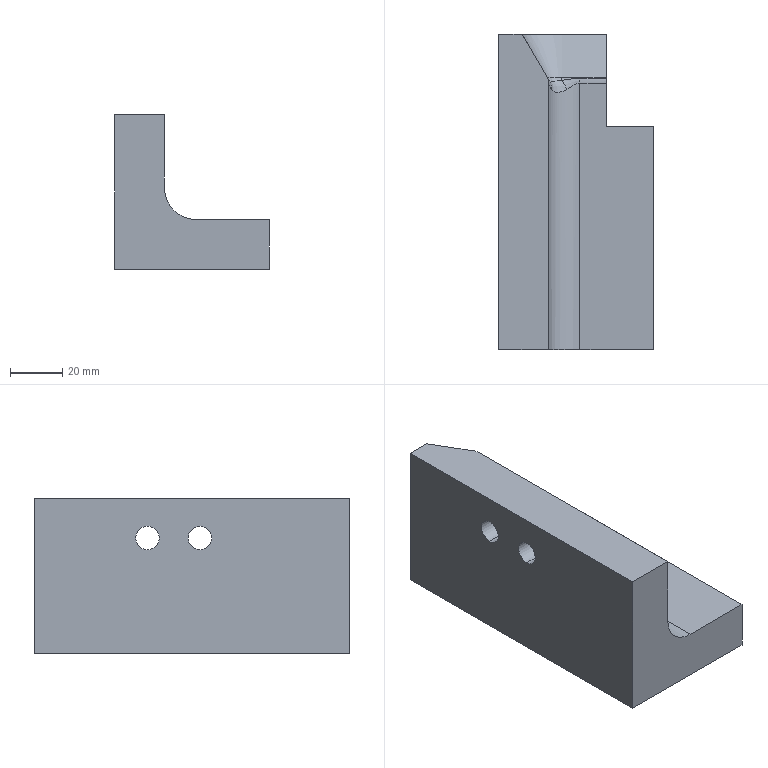Part | 1 solid | 30 faces | box 59 x 120 x 59.001 mm | volume 206950 mm3 | cylinder 13 | plane 12 | spline 5 | commonest cylinder face diameters 9 x4 15 x4 4 x2 10 x2 24 x1
STEP:
#1=CARTESIAN_POINT('',(-19.,-25.,120.5));
#2=VERTEX_POINT('',#1);
#3=CARTESIAN_POINT('',(-19.,-25.,105.5));
#4=VERTEX_POINT('',#3);
#5=CARTESIAN_POINT('',(-19.,-25.,113.));
#6=DIRECTION('',(-1.,0.,0.));
#7=DIRECTION('',(0.,0.,1.));
#8=AXIS2_PLACEMENT_3D('',#5,#6,#7);
#9=CIRCLE('',#8,7.5);
#10=EDGE_CURVE('',#2,#4,#9,.T.);
#11=ORIENTED_EDGE('',*,*,#10,.T.);
#12=CARTESIAN_POINT('',(-10.,-25.,105.5));
#13=VERTEX_POINT('',#12);
#14=CARTESIAN_POINT('',(-10.,-25.,105.5));
#15=DIRECTION('',(1.,0.,0.));
#16=VECTOR('',#15,1000.);
#17=LINE('',#14,#16);
#18=EDGE_CURVE('',#4,#13,#17,.T.);
#19=ORIENTED_EDGE('',*,*,#18,.T.);
#20=CARTESIAN_POINT('',(-10.,-25.,120.5));
#21=VERTEX_POINT('',#20);
#22=CARTESIAN_POINT('',(-10.,-25.,113.));
#23=DIRECTION('',(-1.,0.,0.));
#24=DIRECTION('',(0.,0.,1.));
#25=AXIS2_PLACEMENT_3D('',#22,#23,#24);
#26=CIRCLE('',#25,7.5);
#27=EDGE_CURVE('',#21,#13,#26,.T.);
#28=ORIENTED_EDGE('',*,*,#27,.F.);
#29=CARTESIAN_POINT('',(-10.,-25.,120.5));
#30=DIRECTION('',(1.,0.,0.));
#31=VECTOR('',#30,1000.);
#32=LINE('',#29,#31);
#33=EDGE_CURVE('',#2,#21,#32,.T.);
#34=ORIENTED_EDGE('',*,*,#33,.F.);
#35=EDGE_LOOP('',(#11,#19,#28,#34));
#36=FACE_OUTER_BOUND('',#35,.T.);
#37=CARTESIAN_POINT('',(-10.,-25.,113.));
#38=DIRECTION('',(1.,0.,0.));
#39=DIRECTION('',(0.,0.,1.));
#40=AXIS2_PLACEMENT_3D('',#37,#38,#39);
#41=CYLINDRICAL_SURFACE('',#40,7.5);
#42=ADVANCED_FACE('',(#36),#41,.F.);
#43=CARTESIAN_POINT('',(-19.,-45.,120.5));
#44=VERTEX_POINT('',#43);
#45=CARTESIAN_POINT('',(-19.,-45.,105.5));
#46=VERTEX_POINT('',#45);
#47=CARTESIAN_POINT('',(-19.,-45.,113.));
#48=DIRECTION('',(-1.,0.,0.));
#49=DIRECTION('',(0.,0.,1.));
#50=AXIS2_PLACEMENT_3D('',#47,#48,#49);
#51=CIRCLE('',#50,7.5);
#52=EDGE_CURVE('',#44,#46,#51,.T.);
#53=ORIENTED_EDGE('',*,*,#52,.T.);
#54=CARTESIAN_POINT('',(-10.,-45.,105.5));
#55=VERTEX_POINT('',#54);
#56=CARTESIAN_POINT('',(-10.,-45.,105.5));
#57=DIRECTION('',(1.,0.,0.));
#58=VECTOR('',#57,1000.);
#59=LINE('',#56,#58);
#60=EDGE_CURVE('',#46,#55,#59,.T.);
#61=ORIENTED_EDGE('',*,*,#60,.T.);
#62=CARTESIAN_POINT('',(-10.,-45.,120.5));
#63=VERTEX_POINT('',#62);
#64=CARTESIAN_POINT('',(-10.,-45.,113.));
#65=DIRECTION('',(-1.,0.,0.));
#66=DIRECTION('',(0.,0.,1.));
#67=AXIS2_PLACEMENT_3D('',#64,#65,#66);
#68=CIRCLE('',#67,7.5);
#69=EDGE_CURVE('',#63,#55,#68,.T.);
#70=ORIENTED_EDGE('',*,*,#69,.F.);
#71=CARTESIAN_POINT('',(-10.,-45.,120.5));
#72=DIRECTION('',(1.,0.,0.));
#73=VECTOR('',#72,1000.);
#74=LINE('',#71,#73);
#75=EDGE_CURVE('',#44,#63,#74,.T.);
#76=ORIENTED_EDGE('',*,*,#75,.F.);
#77=EDGE_LOOP('',(#53,#61,#70,#76));
#78=FACE_OUTER_BOUND('',#77,.T.);
#79=CARTESIAN_POINT('',(-10.,-45.,113.));
#80=DIRECTION('',(1.,0.,0.));
#81=DIRECTION('',(0.,0.,1.));
#82=AXIS2_PLACEMENT_3D('',#79,#80,#81);
#83=CYLINDRICAL_SURFACE('',#82,7.5);
#84=ADVANCED_FACE('',(#78),#83,.F.);
#85=CARTESIAN_POINT('',(-29.,-25.,117.5));
#86=VERTEX_POINT('',#85);
#87=CARTESIAN_POINT('',(-29.,-25.,108.5));
#88=VERTEX_POINT('',#87);
#89=CARTESIAN_POINT('',(-29.,-25.,113.));
#90=DIRECTION('',(-1.,0.,0.));
#91=DIRECTION('',(0.,0.,-1.));
#92=AXIS2_PLACEMENT_3D('',#89,#90,#91);
#93=CIRCLE('',#92,4.5);
#94=EDGE_CURVE('',#86,#88,#93,.T.);
#95=ORIENTED_EDGE('',*,*,#94,.T.);
#96=CARTESIAN_POINT('',(-19.,-25.,108.5));
#97=VERTEX_POINT('',#96);
#98=CARTESIAN_POINT('',(-10.,-25.,108.5));
#99=DIRECTION('',(1.,0.,0.));
#100=VECTOR('',#99,1000.);
#101=LINE('',#98,#100);
#102=EDGE_CURVE('',#88,#97,#101,.T.);
#103=ORIENTED_EDGE('',*,*,#102,.T.);
#104=CARTESIAN_POINT('',(-19.,-25.,117.5));
#105=VERTEX_POINT('',#104);
#106=CARTESIAN_POINT('',(-19.,-25.,113.));
#107=DIRECTION('',(-1.,0.,0.));
#108=DIRECTION('',(0.,0.,1.));
#109=AXIS2_PLACEMENT_3D('',#106,#107,#108);
#110=CIRCLE('',#109,4.5);
#111=EDGE_CURVE('',#105,#97,#110,.T.);
#112=ORIENTED_EDGE('',*,*,#111,.F.);
#113=CARTESIAN_POINT('',(-10.,-25.,117.5));
#114=DIRECTION('',(1.,0.,0.));
#115=VECTOR('',#114,1000.);
#116=LINE('',#113,#115);
#117=EDGE_CURVE('',#86,#105,#116,.T.);
#118=ORIENTED_EDGE('',*,*,#117,.F.);
#119=EDGE_LOOP('',(#95,#103,#112,#118));
#120=FACE_OUTER_BOUND('',#119,.T.);
#121=CARTESIAN_POINT('',(-10.,-25.,113.));
#122=DIRECTION('',(1.,0.,0.));
#123=DIRECTION('',(0.,0.,1.));
#124=AXIS2_PLACEMENT_3D('',#121,#122,#123);
#125=CYLINDRICAL_SURFACE('',#124,4.5);
#126=ADVANCED_FACE('',(#120),#125,.F.);
#127=CARTESIAN_POINT('',(-29.,-45.,117.5));
#128=VERTEX_POINT('',#127);
#129=CARTESIAN_POINT('',(-29.,-45.,108.5));
#130=VERTEX_POINT('',#129);
#131=CARTESIAN_POINT('',(-29.,-45.,113.));
#132=DIRECTION('',(-1.,0.,0.));
#133=DIRECTION('',(0.,0.,-1.));
#134=AXIS2_PLACEMENT_3D('',#131,#132,#133);
#135=CIRCLE('',#134,4.5);
#136=EDGE_CURVE('',#128,#130,#135,.T.);
#137=ORIENTED_EDGE('',*,*,#136,.T.);
#138=CARTESIAN_POINT('',(-19.,-45.,108.5));
#139=VERTEX_POINT('',#138);
#140=CARTESIAN_POINT('',(-10.,-45.,108.5));
#141=DIRECTION('',(1.,0.,0.));
#142=VECTOR('',#141,1000.);
#143=LINE('',#140,#142);
#144=EDGE_CURVE('',#130,#139,#143,.T.);
#145=ORIENTED_EDGE('',*,*,#144,.T.);
#146=CARTESIAN_POINT('',(-19.,-45.,117.5));
#147=VERTEX_POINT('',#146);
#148=CARTESIAN_POINT('',(-19.,-45.,113.));
#149=DIRECTION('',(-1.,0.,0.));
#150=DIRECTION('',(0.,0.,1.));
#151=AXIS2_PLACEMENT_3D('',#148,#149,#150);
#152=CIRCLE('',#151,4.5);
#153=EDGE_CURVE('',#147,#139,#152,.T.);
#154=ORIENTED_EDGE('',*,*,#153,.F.);
#155=CARTESIAN_POINT('',(-10.,-45.,117.5));
#156=DIRECTION('',(1.,0.,0.));
#157=VECTOR('',#156,1000.);
#158=LINE('',#155,#157);
#159=EDGE_CURVE('',#128,#147,#158,.T.);
#160=ORIENTED_EDGE('',*,*,#159,.F.);
#161=EDGE_LOOP('',(#137,#145,#154,#160));
#162=FACE_OUTER_BOUND('',#161,.T.);
#163=CARTESIAN_POINT('',(-10.,-45.,113.));
#164=DIRECTION('',(1.,0.,0.));
#165=DIRECTION('',(0.,0.,1.));
#166=AXIS2_PLACEMENT_3D('',#163,#164,#165);
#167=CYLINDRICAL_SURFACE('',#166,4.5);
#168=ADVANCED_FACE('',(#162),#167,.F.);
#169=CARTESIAN_POINT('',(-29.,-102.,69.));
#170=VERTEX_POINT('',#169);
#171=CARTESIAN_POINT('',(30.,-102.,69.));
#172=VERTEX_POINT('',#171);
#173=CARTESIAN_POINT('',(-30.,-102.,69.));
#174=DIRECTION('',(1.,0.,0.));
#175=VECTOR('',#174,1000.);
#176=LINE('',#173,#175);
#177=EDGE_CURVE('',#170,#172,#176,.T.);
#178=ORIENTED_EDGE('',*,*,#177,.T.);
#179=CARTESIAN_POINT('',(30.,-102.,88.));
#180=VERTEX_POINT('',#179);
#181=CARTESIAN_POINT('',(30.,-102.,88.));
#182=DIRECTION('',(0.,0.,-1.));
#183=VECTOR('',#182,1000.);
#184=LINE('',#181,#183);
#185=EDGE_CURVE('',#180,#172,#184,.T.);
#186=ORIENTED_EDGE('',*,*,#185,.F.);
#187=CARTESIAN_POINT('',(2.,-102.,88.));
#188=VERTEX_POINT('',#187);
#189=CARTESIAN_POINT('',(2.,-102.,88.));
#190=DIRECTION('',(1.,0.,0.));
#191=VECTOR('',#190,1000.);
#192=LINE('',#189,#191);
#193=EDGE_CURVE('',#188,#180,#192,.T.);
#194=ORIENTED_EDGE('',*,*,#193,.F.);
#195=CARTESIAN_POINT('',(-10.,-102.,100.));
#196=VERTEX_POINT('',#195);
#197=CARTESIAN_POINT('',(2.,-102.,100.));
#198=DIRECTION('',(0.,-1.,0.));
#199=DIRECTION('',(0.,0.,1.));
#200=AXIS2_PLACEMENT_3D('',#197,#198,#199);
#201=CIRCLE('',#200,12.);
#202=EDGE_CURVE('',#196,#188,#201,.T.);
#203=ORIENTED_EDGE('',*,*,#202,.F.);
#204=CARTESIAN_POINT('',(-10.,-102.,128.));
#205=VERTEX_POINT('',#204);
#206=CARTESIAN_POINT('',(-10.,-102.,128.));
#207=DIRECTION('',(0.,0.,-1.));
#208=VECTOR('',#207,1000.);
#209=LINE('',#206,#208);
#210=EDGE_CURVE('',#205,#196,#209,.T.);
#211=ORIENTED_EDGE('',*,*,#210,.F.);
#212=CARTESIAN_POINT('',(-29.,-102.,128.));
#213=VERTEX_POINT('',#212);
#214=CARTESIAN_POINT('',(-30.,-102.,128.));
#215=DIRECTION('',(1.,0.,0.));
#216=VECTOR('',#215,1000.);
#217=LINE('',#214,#216);
#218=EDGE_CURVE('',#213,#205,#217,.T.);
#219=ORIENTED_EDGE('',*,*,#218,.F.);
#220=CARTESIAN_POINT('',(-29.,-102.,128.));
#221=DIRECTION('',(0.,0.,-1.));
#222=VECTOR('',#221,1000.);
#223=LINE('',#220,#222);
#224=EDGE_CURVE('',#213,#170,#223,.T.);
#225=ORIENTED_EDGE('',*,*,#224,.T.);
#226=EDGE_LOOP('',(#178,#186,#194,#203,#211,#219,#225));
#227=FACE_OUTER_BOUND('',#226,.T.);
#228=CARTESIAN_POINT('',(2.,-102.,100.));
#229=DIRECTION('',(0.,-1.,0.));
#230=DIRECTION('',(0.,0.,1.));
#231=AXIS2_PLACEMENT_3D('',#228,#229,#230);
#232=PLANE('',#231);
#233=ADVANCED_FACE('',(#227),#232,.T.);
#234=CARTESIAN_POINT('',(-20.,18.,128.));
#235=VERTEX_POINT('',#234);
#236=CARTESIAN_POINT('',(-20.,18.,93.));
#237=VERTEX_POINT('',#236);
#238=CARTESIAN_POINT('',(-20.,18.,128.));
#239=DIRECTION('',(0.,0.,-1.));
#240=VECTOR('',#239,1000.);
#241=LINE('',#238,#240);
#242=EDGE_CURVE('',#235,#237,#241,.T.);
#243=ORIENTED_EDGE('',*,*,#242,.T.);
#244=CARTESIAN_POINT('',(-5.,18.,78.));
#245=VERTEX_POINT('',#244);
#246=CARTESIAN_POINT('',(-5.,18.,93.));
#247=DIRECTION('',(0.,-1.,0.));
#248=DIRECTION('',(0.,0.,-1.));
#249=AXIS2_PLACEMENT_3D('',#246,#247,#248);
#250=CIRCLE('',#249,15.);
#251=EDGE_CURVE('',#237,#245,#250,.T.);
#252=ORIENTED_EDGE('',*,*,#251,.T.);
#253=CARTESIAN_POINT('',(12.,18.,78.));
#254=VERTEX_POINT('',#253);
#255=CARTESIAN_POINT('',(-5.,18.,78.));
#256=DIRECTION('',(1.,0.,0.));
#257=VECTOR('',#256,1000.);
#258=LINE('',#255,#257);
#259=EDGE_CURVE('',#245,#254,#258,.T.);
#260=ORIENTED_EDGE('',*,*,#259,.T.);
#261=CARTESIAN_POINT('',(12.,18.,69.));
#262=VERTEX_POINT('',#261);
#263=CARTESIAN_POINT('',(12.,18.,98.));
#264=DIRECTION('',(0.,0.,-1.));
#265=VECTOR('',#264,1000.);
#266=LINE('',#263,#265);
#267=EDGE_CURVE('',#254,#262,#266,.T.);
#268=ORIENTED_EDGE('',*,*,#267,.T.);
#269=CARTESIAN_POINT('',(-29.,18.,69.));
#270=VERTEX_POINT('',#269);
#271=CARTESIAN_POINT('',(12.,18.,69.));
#272=DIRECTION('',(-1.,0.,0.));
#273=VECTOR('',#272,1000.);
#274=LINE('',#271,#273);
#275=EDGE_CURVE('',#262,#270,#274,.T.);
#276=ORIENTED_EDGE('',*,*,#275,.T.);
#277=CARTESIAN_POINT('',(-29.,18.,128.));
#278=VERTEX_POINT('',#277);
#279=CARTESIAN_POINT('',(-29.,18.,69.));
#280=DIRECTION('',(0.,0.,1.));
#281=VECTOR('',#280,1000.);
#282=LINE('',#279,#281);
#283=EDGE_CURVE('',#270,#278,#282,.T.);
#284=ORIENTED_EDGE('',*,*,#283,.T.);
#285=CARTESIAN_POINT('',(-30.,18.,128.));
#286=DIRECTION('',(-1.,0.,0.));
#287=VECTOR('',#286,1000.);
#288=LINE('',#285,#287);
#289=EDGE_CURVE('',#235,#278,#288,.T.);
#290=ORIENTED_EDGE('',*,*,#289,.F.);
#291=EDGE_LOOP('',(#243,#252,#260,#268,#276,#284,#290));
#292=FACE_OUTER_BOUND('',#291,.T.);
#293=CARTESIAN_POINT('',(0.,18.,98.));
#294=DIRECTION('',(0.,1.,0.));
#295=DIRECTION('',(0.,0.,-1.));
#296=AXIS2_PLACEMENT_3D('',#293,#294,#295);
#297=PLANE('',#296);
#298=ADVANCED_FACE('',(#292),#297,.T.);
#299=ORIENTED_EDGE('',*,*,#289,.T.);
#300=CARTESIAN_POINT('',(-29.,18.,128.));
#301=DIRECTION('',(0.,-1.,0.));
#302=VECTOR('',#301,1000.);
#303=LINE('',#300,#302);
#304=EDGE_CURVE('',#278,#213,#303,.T.);
#305=ORIENTED_EDGE('',*,*,#304,.T.);
#306=ORIENTED_EDGE('',*,*,#218,.T.);
#307=CARTESIAN_POINT('',(-10.,-0.4384,128.));
#308=VERTEX_POINT('',#307);
#309=CARTESIAN_POINT('',(-10.,40.,128.));
#310=DIRECTION('',(0.,-1.,0.));
#311=VECTOR('',#310,1000.);
#312=LINE('',#309,#311);
#313=EDGE_CURVE('',#308,#205,#312,.T.);
#314=ORIENTED_EDGE('',*,*,#313,.F.);
#315=CARTESIAN_POINT('',(-10.313,1.303,128.));
#316=VERTEX_POINT('',#315);
#317=CARTESIAN_POINT('',(-15.,-0.4384,128.));
#318=DIRECTION('',(0.,0.,-1.));
#319=DIRECTION('',(1.,0.,0.));
#320=AXIS2_PLACEMENT_3D('',#317,#318,#319);
#321=CIRCLE('',#320,5.);
#322=EDGE_CURVE('',#316,#308,#321,.T.);
#323=ORIENTED_EDGE('',*,*,#322,.F.);
#324=CARTESIAN_POINT('',(-10.378,1.51,128.001));
#325=VERTEX_POINT('',#324);
#326=CARTESIAN_POINT('',(-8.438,2.,128.));
#327=DIRECTION('',(0.,0.,1.));
#328=DIRECTION('',(1.,0.,0.));
#329=AXIS2_PLACEMENT_3D('',#326,#327,#328);
#330=CIRCLE('',#329,2.);
#331=EDGE_CURVE('',#325,#316,#330,.T.);
#332=ORIENTED_EDGE('',*,*,#331,.F.);
#333=CARTESIAN_POINT('',(-20.,18.,128.));
#334=CARTESIAN_POINT('',(-19.195,16.621,128.));
#335=CARTESIAN_POINT('',(-18.39,15.241,128.));
#336=CARTESIAN_POINT('',(-17.586,13.862,128.));
#337=CARTESIAN_POINT('',(-16.781,12.482,128.));
#338=CARTESIAN_POINT('',(-15.976,11.103,128.));
#339=CARTESIAN_POINT('',(-15.171,9.724,128.));
#340=CARTESIAN_POINT('',(-13.574,6.986,128.));
#341=CARTESIAN_POINT('',(-11.976,4.248,128.));
#342=CARTESIAN_POINT('',(-10.378,1.51,128.001));
#343=B_SPLINE_CURVE_WITH_KNOTS('',3,(#333,#334,#335,#336,#337,#338,#339,#340,#341,#342),.UNSPECIFIED.,.F.,.F.,(4,3,3,4),(0.,0.004791,0.009582,0.01909),.UNSPECIFIED.);
#344=EDGE_CURVE('',#235,#325,#343,.T.);
#345=ORIENTED_EDGE('',*,*,#344,.F.);
#346=EDGE_LOOP('',(#299,#305,#306,#314,#323,#332,#345));
#347=FACE_OUTER_BOUND('',#346,.T.);
#348=CARTESIAN_POINT('',(-10.,40.,128.));
#349=DIRECTION('',(0.,0.,-1.));
#350=DIRECTION('',(1.,0.,0.));
#351=AXIS2_PLACEMENT_3D('',#348,#349,#350);
#352=PLANE('',#351);
#353=ADVANCED_FACE('',(#347),#352,.F.);
#354=ORIENTED_EDGE('',*,*,#144,.F.);
#355=CARTESIAN_POINT('',(-29.,-45.,113.));
#356=DIRECTION('',(-1.,0.,0.));
#357=DIRECTION('',(0.,0.,-1.));
#358=AXIS2_PLACEMENT_3D('',#355,#356,#357);
#359=CIRCLE('',#358,4.5);
#360=EDGE_CURVE('',#130,#128,#359,.T.);
#361=ORIENTED_EDGE('',*,*,#360,.T.);
#362=ORIENTED_EDGE('',*,*,#159,.T.);
#363=CARTESIAN_POINT('',(-19.,-45.,113.));
#364=DIRECTION('',(-1.,0.,0.));
#365=DIRECTION('',(0.,0.,1.));
#366=AXIS2_PLACEMENT_3D('',#363,#364,#365);
#367=CIRCLE('',#366,4.5);
#368=EDGE_CURVE('',#139,#147,#367,.T.);
#369=ORIENTED_EDGE('',*,*,#368,.F.);
#370=EDGE_LOOP('',(#354,#361,#362,#369));
#371=FACE_OUTER_BOUND('',#370,.T.);
#372=CARTESIAN_POINT('',(-10.,-45.,113.));
#373=DIRECTION('',(1.,0.,0.));
#374=DIRECTION('',(0.,0.,1.));
#375=AXIS2_PLACEMENT_3D('',#372,#373,#374);
#376=CYLINDRICAL_SURFACE('',#375,4.5);
#377=ADVANCED_FACE('',(#371),#376,.F.);
#378=ORIENTED_EDGE('',*,*,#102,.F.);
#379=CARTESIAN_POINT('',(-29.,-25.,113.));
#380=DIRECTION('',(-1.,0.,0.));
#381=DIRECTION('',(0.,0.,-1.));
#382=AXIS2_PLACEMENT_3D('',#379,#380,#381);
#383=CIRCLE('',#382,4.5);
#384=EDGE_CURVE('',#88,#86,#383,.T.);
#385=ORIENTED_EDGE('',*,*,#384,.T.);
#386=ORIENTED_EDGE('',*,*,#117,.T.);
#387=CARTESIAN_POINT('',(-19.,-25.,113.));
#388=DIRECTION('',(-1.,0.,0.));
#389=DIRECTION('',(0.,0.,1.));
#390=AXIS2_PLACEMENT_3D('',#387,#388,#389);
#391=CIRCLE('',#390,4.5);
#392=EDGE_CURVE('',#97,#105,#391,.T.);
#393=ORIENTED_EDGE('',*,*,#392,.F.);
#394=EDGE_LOOP('',(#378,#385,#386,#393));
#395=FACE_OUTER_BOUND('',#394,.T.);
#396=CARTESIAN_POINT('',(-10.,-25.,113.));
#397=DIRECTION('',(1.,0.,0.));
#398=DIRECTION('',(0.,0.,1.));
#399=AXIS2_PLACEMENT_3D('',#396,#397,#398);
#400=CYLINDRICAL_SURFACE('',#399,4.5);
#401=ADVANCED_FACE('',(#395),#400,.F.);
#402=ORIENTED_EDGE('',*,*,#275,.F.);
#403=CARTESIAN_POINT('',(12.,-17.,69.));
#404=VERTEX_POINT('',#403);
#405=CARTESIAN_POINT('',(12.,-17.,69.));
#406=DIRECTION('',(0.,1.,0.));
#407=VECTOR('',#406,1000.);
#408=LINE('',#405,#407);
#409=EDGE_CURVE('',#404,#262,#408,.T.);
#410=ORIENTED_EDGE('',*,*,#409,.F.);
#411=CARTESIAN_POINT('',(30.,-17.,69.));
#412=VERTEX_POINT('',#411);
#413=CARTESIAN_POINT('',(30.,-17.,69.));
#414=DIRECTION('',(-1.,0.,0.));
#415=VECTOR('',#414,1000.);
#416=LINE('',#413,#415);
#417=EDGE_CURVE('',#412,#404,#416,.T.);
#418=ORIENTED_EDGE('',*,*,#417,.F.);
#419=CARTESIAN_POINT('',(30.,-102.,69.));
#420=DIRECTION('',(0.,1.,0.));
#421=VECTOR('',#420,1000.);
#422=LINE('',#419,#421);
#423=EDGE_CURVE('',#172,#412,#422,.T.);
#424=ORIENTED_EDGE('',*,*,#423,.F.);
#425=ORIENTED_EDGE('',*,*,#177,.F.);
#426=CARTESIAN_POINT('',(-29.,-102.,69.));
#427=DIRECTION('',(0.,1.,0.));
#428=VECTOR('',#427,1000.);
#429=LINE('',#426,#428);
#430=EDGE_CURVE('',#170,#270,#429,.T.);
#431=ORIENTED_EDGE('',*,*,#430,.T.);
#432=EDGE_LOOP('',(#402,#410,#418,#424,#425,#431));
#433=FACE_OUTER_BOUND('',#432,.T.);
#434=CARTESIAN_POINT('',(0.,0.,69.));
#435=DIRECTION('',(0.,0.,-1.));
#436=DIRECTION('',(1.,0.,0.));
#437=AXIS2_PLACEMENT_3D('',#434,#435,#436);
#438=PLANE('',#437);
#439=ADVANCED_FACE('',(#433),#438,.T.);
#440=ORIENTED_EDGE('',*,*,#423,.T.);
#441=CARTESIAN_POINT('',(30.,-17.,88.));
#442=VERTEX_POINT('',#441);
#443=CARTESIAN_POINT('',(30.,-17.,105.));
#444=DIRECTION('',(0.,0.,-1.));
#445=VECTOR('',#444,1000.);
#446=LINE('',#443,#445);
#447=EDGE_CURVE('',#442,#412,#446,.T.);
#448=ORIENTED_EDGE('',*,*,#447,.F.);
#449=CARTESIAN_POINT('',(30.,40.,88.));
#450=DIRECTION('',(0.,-1.,0.));
#451=VECTOR('',#450,1000.);
#452=LINE('',#449,#451);
#453=EDGE_CURVE('',#442,#180,#452,.T.);
#454=ORIENTED_EDGE('',*,*,#453,.T.);
#455=ORIENTED_EDGE('',*,*,#185,.T.);
#456=EDGE_LOOP('',(#440,#448,#454,#455));
#457=FACE_OUTER_BOUND('',#456,.T.);
#458=CARTESIAN_POINT('',(30.,40.,68.));
#459=DIRECTION('',(-1.,0.,0.));
#460=DIRECTION('',(0.,0.,-1.));
#461=AXIS2_PLACEMENT_3D('',#458,#459,#460);
#462=PLANE('',#461);
#463=ADVANCED_FACE('',(#457),#462,.F.);
#464=ORIENTED_EDGE('',*,*,#417,.T.);
#465=CARTESIAN_POINT('',(12.,-17.,88.));
#466=VERTEX_POINT('',#465);
#467=CARTESIAN_POINT('',(12.,-17.,105.));
#468=DIRECTION('',(0.,0.,-1.));
#469=VECTOR('',#468,1000.);
#470=LINE('',#467,#469);
#471=EDGE_CURVE('',#466,#404,#470,.T.);
#472=ORIENTED_EDGE('',*,*,#471,.F.);
#473=CARTESIAN_POINT('',(30.,-17.,88.));
#474=DIRECTION('',(1.,0.,0.));
#475=VECTOR('',#474,1000.);
#476=LINE('',#473,#475);
#477=EDGE_CURVE('',#466,#442,#476,.T.);
#478=ORIENTED_EDGE('',*,*,#477,.T.);
#479=ORIENTED_EDGE('',*,*,#447,.T.);
#480=EDGE_LOOP('',(#464,#472,#478,#479));
#481=FACE_OUTER_BOUND('',#480,.T.);
#482=CARTESIAN_POINT('',(30.,-17.,105.));
#483=DIRECTION('',(0.,-1.,0.));
#484=DIRECTION('',(1.,0.,0.));
#485=AXIS2_PLACEMENT_3D('',#482,#483,#484);
#486=PLANE('',#485);
#487=ADVANCED_FACE('',(#481),#486,.F.);
#488=CARTESIAN_POINT('',(12.,1.51,87.623));
#489=VERTEX_POINT('',#488);
#490=CARTESIAN_POINT('',(12.,1.303,87.687));
#491=VERTEX_POINT('',#490);
#492=CARTESIAN_POINT('',(12.,2.,89.562));
#493=DIRECTION('',(-1.,0.,0.));
#494=DIRECTION('',(0.,-1.,0.));
#495=AXIS2_PLACEMENT_3D('',#492,#493,#494);
#496=CIRCLE('',#495,2.);
#497=EDGE_CURVE('',#489,#491,#496,.T.);
#498=ORIENTED_EDGE('',*,*,#497,.T.);
#499=CARTESIAN_POINT('',(12.,-0.4384,88.));
#500=VERTEX_POINT('',#499);
#501=CARTESIAN_POINT('',(12.,-0.4384,83.));
#502=DIRECTION('',(-1.,0.,0.));
#503=DIRECTION('',(0.,-1.,0.));
#504=AXIS2_PLACEMENT_3D('',#501,#502,#503);
#505=CIRCLE('',#504,5.);
#506=EDGE_CURVE('',#500,#491,#505,.T.);
#507=ORIENTED_EDGE('',*,*,#506,.F.);
#508=CARTESIAN_POINT('',(12.,40.,88.));
#509=DIRECTION('',(0.,-1.,0.));
#510=VECTOR('',#509,1000.);
#511=LINE('',#508,#510);
#512=EDGE_CURVE('',#500,#466,#511,.T.);
#513=ORIENTED_EDGE('',*,*,#512,.T.);
#514=ORIENTED_EDGE('',*,*,#471,.T.);
#515=ORIENTED_EDGE('',*,*,#409,.T.);
#516=ORIENTED_EDGE('',*,*,#267,.F.);
#517=CARTESIAN_POINT('',(12.,18.,78.));
#518=CARTESIAN_POINT('',(12.,12.503,81.207));
#519=CARTESIAN_POINT('',(12.,7.007,84.414));
#520=CARTESIAN_POINT('',(12.,1.51,87.623));
#521=B_SPLINE_CURVE_WITH_KNOTS('',3,(#517,#518,#519,#520),.UNSPECIFIED.,.F.,.F.,(4,4),(0.,1.),.UNSPECIFIED.);
#522=EDGE_CURVE('',#254,#489,#521,.T.);
#523=ORIENTED_EDGE('',*,*,#522,.T.);
#524=EDGE_LOOP('',(#498,#507,#513,#514,#515,#516,#523));
#525=FACE_OUTER_BOUND('',#524,.T.);
#526=CARTESIAN_POINT('',(12.,-17.,105.));
#527=DIRECTION('',(-1.,0.,0.));
#528=DIRECTION('',(0.,-1.,0.));
#529=AXIS2_PLACEMENT_3D('',#526,#527,#528);
#530=PLANE('',#529);
#531=ADVANCED_FACE('',(#525),#530,.F.);
#532=CARTESIAN_POINT('',(-10.,-0.4384,100.));
#533=VERTEX_POINT('',#532);
#534=CARTESIAN_POINT('',(-10.,40.,100.));
#535=DIRECTION('',(0.,-1.,0.));
#536=VECTOR('',#535,1000.);
#537=LINE('',#534,#536);
#538=EDGE_CURVE('',#533,#196,#537,.T.);
#539=ORIENTED_EDGE('',*,*,#538,.T.);
#540=ORIENTED_EDGE('',*,*,#202,.T.);
#541=CARTESIAN_POINT('',(2.,-0.4384,88.));
#542=VERTEX_POINT('',#541);
#543=CARTESIAN_POINT('',(2.,40.,88.));
#544=DIRECTION('',(0.,-1.,0.));
#545=VECTOR('',#544,1000.);
#546=LINE('',#543,#545);
#547=EDGE_CURVE('',#542,#188,#546,.T.);
#548=ORIENTED_EDGE('',*,*,#547,.F.);
#549=CARTESIAN_POINT('',(-2.941,-2.844,89.065));
#550=VERTEX_POINT('',#549);
#551=CARTESIAN_POINT('',(-2.941,-2.844,89.065));
#552=CARTESIAN_POINT('',(-2.488,-2.541,88.86));
#553=CARTESIAN_POINT('',(-2.061,-2.252,88.7));
#554=CARTESIAN_POINT('',(-1.226,-1.707,88.434));
#555=CARTESIAN_POINT('',(-0.8172,-1.449,88.328));
#556=CARTESIAN_POINT('',(0.3908,-0.7712,88.08));
#557=CARTESIAN_POINT('',(1.177,-0.4384,88.));
#558=CARTESIAN_POINT('',(2.,-0.4384,88.));
#559=B_SPLINE_CURVE_WITH_KNOTS('',3,(#551,#552,#553,#554,#555,#556,#557,#558),.UNSPECIFIED.,.F.,.F.,(4,2,2,4),(0.,0.25,0.5,1.),.UNSPECIFIED.);
#560=EDGE_CURVE('',#550,#542,#559,.T.);
#561=ORIENTED_EDGE('',*,*,#560,.F.);
#562=CARTESIAN_POINT('',(-8.935,-2.844,95.059));
#563=VERTEX_POINT('',#562);
#564=CARTESIAN_POINT('',(-8.935,-2.844,95.059));
#565=CARTESIAN_POINT('',(-8.801,-3.042,94.762));
#566=CARTESIAN_POINT('',(-8.65,-3.21,94.46));
#567=CARTESIAN_POINT('',(-8.31,-3.493,93.85));
#568=CARTESIAN_POINT('',(-8.12,-3.61,93.54));
#569=CARTESIAN_POINT('',(-7.705,-3.792,92.933));
#570=CARTESIAN_POINT('',(-7.483,-3.857,92.637));
#571=CARTESIAN_POINT('',(-7.007,-3.944,92.062));
#572=CARTESIAN_POINT('',(-6.755,-3.966,91.784));
#573=CARTESIAN_POINT('',(-6.216,-3.966,91.246));
#574=CARTESIAN_POINT('',(-5.938,-3.944,90.993));
#575=CARTESIAN_POINT('',(-5.362,-3.857,90.517));
#576=CARTESIAN_POINT('',(-5.066,-3.791,90.294));
#577=CARTESIAN_POINT('',(-4.456,-3.608,89.878));
#578=CARTESIAN_POINT('',(-4.149,-3.492,89.689));
#579=CARTESIAN_POINT('',(-3.54,-3.209,89.35));
#580=CARTESIAN_POINT('',(-3.238,-3.042,89.199));
#581=CARTESIAN_POINT('',(-2.941,-2.844,89.065));
#582=B_SPLINE_CURVE_WITH_KNOTS('',3,(#564,#565,#566,#567,#568,#569,#570,#571,#572,#573,#574,#575,#576,#577,#578,#579,#580,#581),.UNSPECIFIED.,.F.,.F.,(4,2,2,2,2,2,2,2,4),(0.,0.00113,0.00226,0.00339,0.00452,0.00565,0.00678,0.00791,0.00904),.UNSPECIFIED.);
#583=EDGE_CURVE('',#563,#550,#582,.T.);
#584=ORIENTED_EDGE('',*,*,#583,.F.);
#585=CARTESIAN_POINT('',(-10.,-0.4384,100.));
#586=CARTESIAN_POINT('',(-10.,-0.4384,99.518));
#587=CARTESIAN_POINT('',(-9.972,-0.5512,99.061));
#588=CARTESIAN_POINT('',(-9.869,-0.8956,98.175));
#589=CARTESIAN_POINT('',(-9.796,-1.12,97.757));
#590=CARTESIAN_POINT('',(-9.614,-1.591,96.953));
#591=CARTESIAN_POINT('',(-9.505,-1.841,96.566));
#592=CARTESIAN_POINT('',(-9.25,-2.343,95.804));
#593=CARTESIAN_POINT('',(-9.103,-2.596,95.43));
#594=CARTESIAN_POINT('',(-8.935,-2.844,95.059));
#595=B_SPLINE_CURVE_WITH_KNOTS('',3,(#585,#586,#587,#588,#589,#590,#591,#592,#593,#594),.UNSPECIFIED.,.F.,.F.,(4,2,2,2,4),(0.,0.001413,0.002826,0.004239,0.005652),.UNSPECIFIED.);
#596=EDGE_CURVE('',#533,#563,#595,.T.);
#597=ORIENTED_EDGE('',*,*,#596,.F.);
#598=EDGE_LOOP('',(#539,#540,#548,#561,#584,#597));
#599=FACE_OUTER_BOUND('',#598,.T.);
#600=CARTESIAN_POINT('',(2.,40.,100.));
#601=DIRECTION('',(0.,-1.,0.));
#602=DIRECTION('',(0.,0.,1.));
#603=AXIS2_PLACEMENT_3D('',#600,#601,#602);
#604=CYLINDRICAL_SURFACE('',#603,12.);
#605=ADVANCED_FACE('',(#599),#604,.F.);
#606=ORIENTED_EDGE('',*,*,#512,.F.);
#607=CARTESIAN_POINT('',(30.,-0.4384,88.));
#608=DIRECTION('',(1.,0.,0.));
#609=VECTOR('',#608,1000.);
#610=LINE('',#607,#609);
#611=EDGE_CURVE('',#542,#500,#610,.T.);
#612=ORIENTED_EDGE('',*,*,#611,.F.);
#613=ORIENTED_EDGE('',*,*,#547,.T.);
#614=ORIENTED_EDGE('',*,*,#193,.T.);
#615=ORIENTED_EDGE('',*,*,#453,.F.);
#616=ORIENTED_EDGE('',*,*,#477,.F.);
#617=EDGE_LOOP('',(#606,#612,#613,#614,#615,#616));
#618=FACE_OUTER_BOUND('',#617,.T.);
#619=CARTESIAN_POINT('',(30.,40.,88.));
#620=DIRECTION('',(0.,0.,-1.));
#621=DIRECTION('',(1.,0.,0.));
#622=AXIS2_PLACEMENT_3D('',#619,#620,#621);
#623=PLANE('',#622);
#624=ADVANCED_FACE('',(#618),#623,.F.);
#625=ORIENTED_EDGE('',*,*,#27,.T.);
#626=CARTESIAN_POINT('',(-10.,-25.,113.));
#627=DIRECTION('',(-1.,0.,0.));
#628=DIRECTION('',(0.,0.,1.));
#629=AXIS2_PLACEMENT_3D('',#626,#627,#628);
#630=CIRCLE('',#629,7.5);
#631=EDGE_CURVE('',#13,#21,#630,.T.);
#632=ORIENTED_EDGE('',*,*,#631,.T.);
#633=EDGE_LOOP('',(#625,#632));
#634=FACE_BOUND('',#633,.T.);
#635=ORIENTED_EDGE('',*,*,#69,.T.);
#636=CARTESIAN_POINT('',(-10.,-45.,113.));
#637=DIRECTION('',(-1.,0.,0.));
#638=DIRECTION('',(0.,0.,1.));
#639=AXIS2_PLACEMENT_3D('',#636,#637,#638);
#640=CIRCLE('',#639,7.5);
#641=EDGE_CURVE('',#55,#63,#640,.T.);
#642=ORIENTED_EDGE('',*,*,#641,.T.);
#643=EDGE_LOOP('',(#635,#642));
#644=FACE_BOUND('',#643,.T.);
#645=ORIENTED_EDGE('',*,*,#313,.T.);
#646=ORIENTED_EDGE('',*,*,#210,.T.);
#647=ORIENTED_EDGE('',*,*,#538,.F.);
#648=CARTESIAN_POINT('',(-10.,-0.4384,100.));
#649=DIRECTION('',(0.,0.,-1.));
#650=VECTOR('',#649,1000.);
#651=LINE('',#648,#650);
#652=EDGE_CURVE('',#308,#533,#651,.T.);
#653=ORIENTED_EDGE('',*,*,#652,.F.);
#654=EDGE_LOOP('',(#645,#646,#647,#653));
#655=FACE_OUTER_BOUND('',#654,.T.);
#656=CARTESIAN_POINT('',(-10.,40.,100.));
#657=DIRECTION('',(-1.,0.,0.));
#658=DIRECTION('',(0.,0.,-1.));
#659=AXIS2_PLACEMENT_3D('',#656,#657,#658);
#660=PLANE('',#659);
#661=ADVANCED_FACE('',(#634,#644,#655),#660,.F.);
#662=ORIENTED_EDGE('',*,*,#153,.T.);
#663=ORIENTED_EDGE('',*,*,#368,.T.);
#664=EDGE_LOOP('',(#662,#663));
#665=FACE_BOUND('',#664,.T.);
#666=ORIENTED_EDGE('',*,*,#52,.F.);
#667=CARTESIAN_POINT('',(-19.,-45.,113.));
#668=DIRECTION('',(-1.,0.,0.));
#669=DIRECTION('',(0.,0.,1.));
#670=AXIS2_PLACEMENT_3D('',#667,#668,#669);
#671=CIRCLE('',#670,7.5);
#672=EDGE_CURVE('',#46,#44,#671,.T.);
#673=ORIENTED_EDGE('',*,*,#672,.F.);
#674=EDGE_LOOP('',(#666,#673));
#675=FACE_OUTER_BOUND('',#674,.T.);
#676=CARTESIAN_POINT('',(-19.,-40.5,113.));
#677=DIRECTION('',(-1.,0.,0.));
#678=DIRECTION('',(0.,0.,-1.));
#679=AXIS2_PLACEMENT_3D('',#676,#677,#678);
#680=PLANE('',#679);
#681=ADVANCED_FACE('',(#665,#675),#680,.F.);
#682=ORIENTED_EDGE('',*,*,#60,.F.);
#683=ORIENTED_EDGE('',*,*,#672,.T.);
#684=ORIENTED_EDGE('',*,*,#75,.T.);
#685=ORIENTED_EDGE('',*,*,#641,.F.);
#686=EDGE_LOOP('',(#682,#683,#684,#685));
#687=FACE_OUTER_BOUND('',#686,.T.);
#688=CARTESIAN_POINT('',(-10.,-45.,113.));
#689=DIRECTION('',(1.,0.,0.));
#690=DIRECTION('',(0.,0.,1.));
#691=AXIS2_PLACEMENT_3D('',#688,#689,#690);
#692=CYLINDRICAL_SURFACE('',#691,7.5);
#693=ADVANCED_FACE('',(#687),#692,.F.);
#694=ORIENTED_EDGE('',*,*,#111,.T.);
#695=ORIENTED_EDGE('',*,*,#392,.T.);
#696=EDGE_LOOP('',(#694,#695));
#697=FACE_BOUND('',#696,.T.);
#698=ORIENTED_EDGE('',*,*,#10,.F.);
#699=CARTESIAN_POINT('',(-19.,-25.,113.));
#700=DIRECTION('',(-1.,0.,0.));
#701=DIRECTION('',(0.,0.,1.));
#702=AXIS2_PLACEMENT_3D('',#699,#700,#701);
#703=CIRCLE('',#702,7.5);
#704=EDGE_CURVE('',#4,#2,#703,.T.);
#705=ORIENTED_EDGE('',*,*,#704,.F.);
#706=EDGE_LOOP('',(#698,#705));
#707=FACE_OUTER_BOUND('',#706,.T.);
#708=CARTESIAN_POINT('',(-19.,-20.5,113.));
#709=DIRECTION('',(-1.,0.,0.));
#710=DIRECTION('',(0.,0.,-1.));
#711=AXIS2_PLACEMENT_3D('',#708,#709,#710);
#712=PLANE('',#711);
#713=ADVANCED_FACE('',(#697,#707),#712,.F.);
#714=ORIENTED_EDGE('',*,*,#18,.F.);
#715=ORIENTED_EDGE('',*,*,#704,.T.);
#716=ORIENTED_EDGE('',*,*,#33,.T.);
#717=ORIENTED_EDGE('',*,*,#631,.F.);
#718=EDGE_LOOP('',(#714,#715,#716,#717));
#719=FACE_OUTER_BOUND('',#718,.T.);
#720=CARTESIAN_POINT('',(-10.,-25.,113.));
#721=DIRECTION('',(1.,0.,0.));
#722=DIRECTION('',(0.,0.,1.));
#723=AXIS2_PLACEMENT_3D('',#720,#721,#722);
#724=CYLINDRICAL_SURFACE('',#723,7.5);
#725=ADVANCED_FACE('',(#719),#724,.F.);
#726=ORIENTED_EDGE('',*,*,#331,.T.);
#727=CARTESIAN_POINT('',(-10.313,1.303,100.));
#728=VERTEX_POINT('',#727);
#729=CARTESIAN_POINT('',(-10.313,1.303,93.));
#730=DIRECTION('',(0.,0.,1.));
#731=VECTOR('',#730,1000.);
#732=LINE('',#729,#731);
#733=EDGE_CURVE('',#728,#316,#732,.T.);
#734=ORIENTED_EDGE('',*,*,#733,.F.);
#735=CARTESIAN_POINT('',(-9.882,0.6161,93.));
#736=VERTEX_POINT('',#735);
#737=CARTESIAN_POINT('',(-9.882,0.6161,93.));
#738=CARTESIAN_POINT('',(-10.032,0.7719,94.157));
#739=CARTESIAN_POINT('',(-10.138,0.9343,95.317));
#740=CARTESIAN_POINT('',(-10.279,1.202,97.65));
#741=CARTESIAN_POINT('',(-10.313,1.303,98.822));
#742=CARTESIAN_POINT('',(-10.313,1.303,100.));
#743=B_SPLINE_CURVE_WITH_KNOTS('',3,(#737,#738,#739,#740,#741,#742),.UNSPECIFIED.,.F.,.F.,(4,2,4),(0.,0.003527,0.007055),.UNSPECIFIED.);
#744=EDGE_CURVE('',#736,#728,#743,.T.);
#745=ORIENTED_EDGE('',*,*,#744,.F.);
#746=CARTESIAN_POINT('',(-10.378,1.512,93.));
#747=VERTEX_POINT('',#746);
#748=CARTESIAN_POINT('',(-9.882,0.6161,93.));
#749=CARTESIAN_POINT('',(-10.122,0.866,93.));
#750=CARTESIAN_POINT('',(-10.295,1.179,93.));
#751=CARTESIAN_POINT('',(-10.378,1.512,93.));
#752=B_SPLINE_CURVE_WITH_KNOTS('',3,(#748,#749,#750,#751),.UNSPECIFIED.,.F.,.F.,(4,4),(0.6084,1.),.UNSPECIFIED.);
#753=EDGE_CURVE('',#736,#747,#752,.T.);
#754=ORIENTED_EDGE('',*,*,#753,.T.);
#755=CARTESIAN_POINT('',(-10.379,1.51,93.));
#756=DIRECTION('',(0.,0.,-1.));
#757=VECTOR('',#756,1000.);
#758=LINE('',#755,#757);
#759=EDGE_CURVE('',#325,#747,#758,.T.);
#760=ORIENTED_EDGE('',*,*,#759,.F.);
#761=EDGE_LOOP('',(#726,#734,#745,#754,#760));
#762=FACE_OUTER_BOUND('',#761,.T.);
#763=CARTESIAN_POINT('',(-8.438,2.,93.));
#764=DIRECTION('',(0.,0.,-1.));
#765=DIRECTION('',(1.,0.,0.));
#766=AXIS2_PLACEMENT_3D('',#763,#764,#765);
#767=CYLINDRICAL_SURFACE('',#766,2.);
#768=ADVANCED_FACE('',(#762),#767,.F.);
#769=CARTESIAN_POINT('',(-5.,0.6161,88.118));
#770=VERTEX_POINT('',#769);
#771=CARTESIAN_POINT('',(-5.,1.512,87.622));
#772=VERTEX_POINT('',#771);
#773=CARTESIAN_POINT('',(-5.,0.6161,88.118));
#774=CARTESIAN_POINT('',(-5.,0.9996,87.75));
#775=CARTESIAN_POINT('',(-5.,1.512,87.622));
#776=(BOUNDED_CURVE()B_SPLINE_CURVE(2,(#773,#774,#775),.UNSPECIFIED.,.F.,.F.)B_SPLINE_CURVE_WITH_KNOTS((3,3),(0.6045,1.),.UNSPECIFIED.)CURVE()GEOMETRIC_REPRESENTATION_ITEM()RATIONAL_B_SPLINE_CURVE((0.8987,0.9162,1.))REPRESENTATION_ITEM(''));
#777=EDGE_CURVE('',#770,#772,#776,.T.);
#778=ORIENTED_EDGE('',*,*,#777,.T.);
#779=CARTESIAN_POINT('',(-5.,1.512,87.622));
#780=CARTESIAN_POINT('',(-5.704,1.515,87.621));
#781=CARTESIAN_POINT('',(-6.408,1.515,87.761));
#782=CARTESIAN_POINT('',(-7.709,1.515,88.3));
#783=CARTESIAN_POINT('',(-8.305,1.515,88.699));
#784=CARTESIAN_POINT('',(-9.301,1.515,89.695));
#785=CARTESIAN_POINT('',(-9.7,1.515,90.291));
#786=CARTESIAN_POINT('',(-10.239,1.515,91.592));
#787=CARTESIAN_POINT('',(-10.379,1.515,92.296));
#788=CARTESIAN_POINT('',(-10.378,1.512,93.));
#789=B_SPLINE_CURVE_WITH_KNOTS('',3,(#779,#780,#781,#782,#783,#784,#785,#786,#787,#788),.UNSPECIFIED.,.F.,.F.,(4,2,2,2,4),(0.,0.25,0.5,0.75,1.),.UNSPECIFIED.);
#790=EDGE_CURVE('',#772,#747,#789,.T.);
#791=ORIENTED_EDGE('',*,*,#790,.T.);
#792=ORIENTED_EDGE('',*,*,#753,.F.);
#793=CARTESIAN_POINT('',(-5.,0.6161,88.118));
#794=CARTESIAN_POINT('',(-5.145,0.5818,88.151));
#795=CARTESIAN_POINT('',(-5.293,0.5516,88.189));
#796=CARTESIAN_POINT('',(-5.582,0.4986,88.273));
#797=CARTESIAN_POINT('',(-5.726,0.4756,88.32));
#798=CARTESIAN_POINT('',(-6.153,0.4143,88.476));
#799=CARTESIAN_POINT('',(-6.435,0.3836,88.601));
#800=CARTESIAN_POINT('',(-7.245,0.3137,89.033));
#801=CARTESIAN_POINT('',(-7.735,0.2955,89.393));
#802=CARTESIAN_POINT('',(-8.608,0.2955,90.266));
#803=CARTESIAN_POINT('',(-8.967,0.3138,90.756));
#804=CARTESIAN_POINT('',(-9.398,0.3835,91.563));
#805=CARTESIAN_POINT('',(-9.523,0.4141,91.846));
#806=CARTESIAN_POINT('',(-9.679,0.4755,92.274));
#807=CARTESIAN_POINT('',(-9.727,0.4986,92.417));
#808=CARTESIAN_POINT('',(-9.811,0.5516,92.707));
#809=CARTESIAN_POINT('',(-9.849,0.5818,92.855));
#810=CARTESIAN_POINT('',(-9.882,0.6161,93.));
#811=B_SPLINE_CURVE_WITH_KNOTS('',3,(#793,#794,#795,#796,#797,#798,#799,#800,#801,#802,#803,#804,#805,#806,#807,#808,#809,#810),.UNSPECIFIED.,.F.,.F.,(4,2,2,2,2,2,2,2,4),(-0.00000006,0.0004588,0.0009177,0.001835,0.003671,0.005506,0.006424,0.006883,0.007342),.UNSPECIFIED.);
#812=EDGE_CURVE('',#770,#736,#811,.T.);
#813=ORIENTED_EDGE('',*,*,#812,.F.);
#814=EDGE_LOOP('',(#778,#791,#792,#813));
#815=FACE_OUTER_BOUND('',#814,.T.);
#816=CARTESIAN_POINT('',(-5.,1.515,87.621));
#817=CARTESIAN_POINT('',(-5.704,1.515,87.621));
#818=CARTESIAN_POINT('',(-6.408,1.515,87.761));
#819=CARTESIAN_POINT('',(-7.709,1.515,88.3));
#820=CARTESIAN_POINT('',(-8.305,1.515,88.699));
#821=CARTESIAN_POINT('',(-9.301,1.515,89.695));
#822=CARTESIAN_POINT('',(-9.7,1.515,90.291));
#823=CARTESIAN_POINT('',(-10.239,1.515,91.592));
#824=CARTESIAN_POINT('',(-10.379,1.515,92.296));
#825=CARTESIAN_POINT('',(-10.379,1.515,93.));
#826=CARTESIAN_POINT('',(-5.,0.,88.));
#827=CARTESIAN_POINT('',(-5.655,0.,88.));
#828=CARTESIAN_POINT('',(-6.309,0.,88.13));
#829=CARTESIAN_POINT('',(-7.518,0.,88.631));
#830=CARTESIAN_POINT('',(-8.073,0.,89.002));
#831=CARTESIAN_POINT('',(-8.998,0.,89.927));
#832=CARTESIAN_POINT('',(-9.369,0.,90.482));
#833=CARTESIAN_POINT('',(-9.87,0.,91.691));
#834=CARTESIAN_POINT('',(-10.,0.,92.345));
#835=CARTESIAN_POINT('',(-10.,0.,93.));
#836=CARTESIAN_POINT('',(-5.,0.,89.562));
#837=CARTESIAN_POINT('',(-5.45,0.,89.562));
#838=CARTESIAN_POINT('',(-5.9,0.,89.651));
#839=CARTESIAN_POINT('',(-6.732,0.,89.996));
#840=CARTESIAN_POINT('',(-7.113,0.,90.25));
#841=CARTESIAN_POINT('',(-7.75,0.,90.887));
#842=CARTESIAN_POINT('',(-8.004,0.,91.268));
#843=CARTESIAN_POINT('',(-8.349,0.,92.1));
#844=CARTESIAN_POINT('',(-8.438,0.,92.55));
#845=CARTESIAN_POINT('',(-8.438,0.,93.));
#846=(BOUNDED_SURFACE()B_SPLINE_SURFACE(2,3,((#816,#817,#818,#819,#820,#821,#822,#823,#824,#825),(#826,#827,#828,#829,#830,#831,#832,#833,#834,#835),(#836,#837,#838,#839,#840,#841,#842,#843,#844,#845)),.UNSPECIFIED.,.F.,.F.,.F.)B_SPLINE_SURFACE_WITH_KNOTS((3,3),(4,2,2,2,4),(0.,1.),(6.283,6.676,7.069,7.461,7.854),.UNSPECIFIED.)GEOMETRIC_REPRESENTATION_ITEM()RATIONAL_B_SPLINE_SURFACE(((1.,1.,1.,1.,1.,1.,1.,1.,1.,1.),(0.7882,0.7882,0.7882,0.7882,0.7882,0.7882,0.7882,0.7882,0.7882,0.7882),(1.,1.,1.,1.,1.,1.,1.,1.,1.,1.)))REPRESENTATION_ITEM('')SURFACE());
#847=ADVANCED_FACE('',(#815),#846,.F.);
#848=ORIENTED_EDGE('',*,*,#777,.F.);
#849=CARTESIAN_POINT('',(2.,1.303,87.687));
#850=VERTEX_POINT('',#849);
#851=CARTESIAN_POINT('',(2.,1.303,87.687));
#852=CARTESIAN_POINT('',(0.8336,1.303,87.687));
#853=CARTESIAN_POINT('',(-0.2797,1.208,87.719));
#854=CARTESIAN_POINT('',(-1.991,1.015,87.82));
#855=CARTESIAN_POINT('',(-2.571,0.941,87.862));
#856=CARTESIAN_POINT('',(-3.753,0.7851,87.97));
#857=CARTESIAN_POINT('',(-4.358,0.7025,88.035));
#858=CARTESIAN_POINT('',(-5.,0.6161,88.118));
#859=B_SPLINE_CURVE_WITH_KNOTS('',3,(#851,#852,#853,#854,#855,#856,#857,#858),.UNSPECIFIED.,.F.,.F.,(4,2,2,4),(0.,0.5,0.75,1.),.UNSPECIFIED.);
#860=EDGE_CURVE('',#850,#770,#859,.T.);
#861=ORIENTED_EDGE('',*,*,#860,.F.);
#862=CARTESIAN_POINT('',(35.,1.303,87.687));
#863=DIRECTION('',(-1.,0.,0.));
#864=VECTOR('',#863,1000.);
#865=LINE('',#862,#864);
#866=EDGE_CURVE('',#491,#850,#865,.T.);
#867=ORIENTED_EDGE('',*,*,#866,.F.);
#868=ORIENTED_EDGE('',*,*,#497,.F.);
#869=CARTESIAN_POINT('',(12.,1.51,87.621));
#870=DIRECTION('',(1.,0.,0.));
#871=VECTOR('',#870,1000.);
#872=LINE('',#869,#871);
#873=EDGE_CURVE('',#772,#489,#872,.T.);
#874=ORIENTED_EDGE('',*,*,#873,.F.);
#875=EDGE_LOOP('',(#848,#861,#867,#868,#874));
#876=FACE_OUTER_BOUND('',#875,.T.);
#877=CARTESIAN_POINT('',(35.,2.,89.562));
#878=DIRECTION('',(1.,0.,0.));
#879=DIRECTION('',(0.,0.,1.));
#880=AXIS2_PLACEMENT_3D('',#877,#878,#879);
#881=CYLINDRICAL_SURFACE('',#880,2.);
#882=ADVANCED_FACE('',(#876),#881,.F.);
#883=ORIENTED_EDGE('',*,*,#506,.T.);
#884=ORIENTED_EDGE('',*,*,#866,.T.);
#885=CARTESIAN_POINT('',(2.,1.303,87.687));
#886=CARTESIAN_POINT('',(2.,0.7474,87.893));
#887=CARTESIAN_POINT('',(2.,0.1546,88.));
#888=CARTESIAN_POINT('',(2.,-0.4384,88.));
#889=B_SPLINE_CURVE_WITH_KNOTS('',3,(#885,#886,#887,#888),.UNSPECIFIED.,.F.,.F.,(4,4),(0.,1.),.UNSPECIFIED.);
#890=EDGE_CURVE('',#850,#542,#889,.T.);
#891=ORIENTED_EDGE('',*,*,#890,.T.);
#892=ORIENTED_EDGE('',*,*,#611,.T.);
#893=EDGE_LOOP('',(#883,#884,#891,#892));
#894=FACE_OUTER_BOUND('',#893,.T.);
#895=CARTESIAN_POINT('',(35.,-0.4384,83.));
#896=DIRECTION('',(1.,0.,0.));
#897=DIRECTION('',(0.,0.,1.));
#898=AXIS2_PLACEMENT_3D('',#895,#896,#897);
#899=CYLINDRICAL_SURFACE('',#898,5.);
#900=ADVANCED_FACE('',(#894),#899,.T.);
#901=ORIENTED_EDGE('',*,*,#890,.F.);
#902=ORIENTED_EDGE('',*,*,#860,.T.);
#903=CARTESIAN_POINT('',(-5.,0.6161,88.118));
#904=CARTESIAN_POINT('',(-3.758,-0.7569,89.434));
#905=CARTESIAN_POINT('',(-2.941,-2.844,89.065));
#906=(BOUNDED_CURVE()B_SPLINE_CURVE(2,(#903,#904,#905),.UNSPECIFIED.,.F.,.F.)B_SPLINE_CURVE_WITH_KNOTS((3,3),(0.,1.),.UNSPECIFIED.)CURVE()GEOMETRIC_REPRESENTATION_ITEM()RATIONAL_B_SPLINE_CURVE((1.,0.9105,1.))REPRESENTATION_ITEM(''));
#907=EDGE_CURVE('',#770,#550,#906,.T.);
#908=ORIENTED_EDGE('',*,*,#907,.T.);
#909=ORIENTED_EDGE('',*,*,#560,.T.);
#910=EDGE_LOOP('',(#901,#902,#908,#909));
#911=FACE_OUTER_BOUND('',#910,.T.);
#912=CARTESIAN_POINT('',(-2.941,-2.844,89.065));
#913=CARTESIAN_POINT('',(-2.488,-2.541,88.86));
#914=CARTESIAN_POINT('',(-2.061,-2.252,88.7));
#915=CARTESIAN_POINT('',(-1.226,-1.707,88.434));
#916=CARTESIAN_POINT('',(-0.8172,-1.449,88.328));
#917=CARTESIAN_POINT('',(0.3908,-0.7712,88.08));
#918=CARTESIAN_POINT('',(1.177,-0.4384,88.));
#919=CARTESIAN_POINT('',(2.,-0.4384,88.));
#920=CARTESIAN_POINT('',(-3.758,-0.7569,89.434));
#921=CARTESIAN_POINT('',(-3.275,-0.6493,89.175));
#922=CARTESIAN_POINT('',(-2.793,-0.5197,88.96));
#923=CARTESIAN_POINT('',(-1.838,-0.2548,88.602));
#924=CARTESIAN_POINT('',(-1.36,-0.1172,88.456));
#925=CARTESIAN_POINT('',(0.05469,0.255,88.116));
#926=CARTESIAN_POINT('',(1.011,0.4606,88.));
#927=CARTESIAN_POINT('',(2.,0.4606,88.));
#928=CARTESIAN_POINT('',(-5.,0.6161,88.118));
#929=CARTESIAN_POINT('',(-4.358,0.7025,88.035));
#930=CARTESIAN_POINT('',(-3.753,0.7851,87.97));
#931=CARTESIAN_POINT('',(-2.571,0.941,87.862));
#932=CARTESIAN_POINT('',(-1.991,1.015,87.82));
#933=CARTESIAN_POINT('',(-0.2797,1.208,87.719));
#934=CARTESIAN_POINT('',(0.8336,1.303,87.687));
#935=CARTESIAN_POINT('',(2.,1.303,87.687));
#936=(BOUNDED_SURFACE()B_SPLINE_SURFACE(2,3,((#912,#913,#914,#915,#916,#917,#918,#919),(#920,#921,#922,#923,#924,#925,#926,#927),(#928,#929,#930,#931,#932,#933,#934,#935)),.UNSPECIFIED.,.F.,.F.,.F.)B_SPLINE_SURFACE_WITH_KNOTS((3,3),(4,2,2,4),(0.,1.),(0.000907,0.002236,0.003565,0.006223),.UNSPECIFIED.)GEOMETRIC_REPRESENTATION_ITEM()RATIONAL_B_SPLINE_SURFACE(((1.,1.,1.,1.,1.,1.,1.,1.),(0.9105,0.9242,0.9352,0.9536,0.961,0.9785,0.9841,0.9842),(1.,1.,1.,1.,1.,1.,1.,1.)))REPRESENTATION_ITEM('')SURFACE());
#937=ADVANCED_FACE('',(#911),#936,.F.);
#938=ORIENTED_EDGE('',*,*,#907,.F.);
#939=ORIENTED_EDGE('',*,*,#812,.T.);
#940=CARTESIAN_POINT('',(-9.882,0.6161,93.));
#941=CARTESIAN_POINT('',(-9.471,0.1865,93.389));
#942=CARTESIAN_POINT('',(-9.17,-0.3492,93.777));
#943=CARTESIAN_POINT('',(-8.845,-1.538,94.484));
#944=CARTESIAN_POINT('',(-8.82,-2.191,94.803));
#945=CARTESIAN_POINT('',(-8.935,-2.844,95.059));
#946=B_SPLINE_CURVE_WITH_KNOTS('',3,(#940,#941,#942,#943,#944,#945),.UNSPECIFIED.,.F.,.F.,(4,2,4),(0.,0.5,1.),.UNSPECIFIED.);
#947=EDGE_CURVE('',#736,#563,#946,.T.);
#948=ORIENTED_EDGE('',*,*,#947,.T.);
#949=ORIENTED_EDGE('',*,*,#583,.T.);
#950=EDGE_LOOP('',(#938,#939,#948,#949));
#951=FACE_OUTER_BOUND('',#950,.T.);
#952=CARTESIAN_POINT('',(-5.,0.6161,88.118));
#953=CARTESIAN_POINT('',(-3.758,-0.7569,89.434));
#954=CARTESIAN_POINT('',(-2.941,-2.844,89.065));
#955=CARTESIAN_POINT('',(-5.252,0.5566,88.175));
#956=CARTESIAN_POINT('',(-3.994,-0.8521,89.569));
#957=CARTESIAN_POINT('',(-3.253,-3.052,89.205));
#958=CARTESIAN_POINT('',(-5.516,0.5078,88.248));
#959=CARTESIAN_POINT('',(-4.23,-0.9225,89.713));
#960=CARTESIAN_POINT('',(-3.565,-3.223,89.362));
#961=CARTESIAN_POINT('',(-6.057,0.4266,88.438));
#962=CARTESIAN_POINT('',(-4.698,-1.032,90.022));
#963=CARTESIAN_POINT('',(-4.183,-3.507,89.71));
#964=CARTESIAN_POINT('',(-6.335,0.3941,88.555));
#965=CARTESIAN_POINT('',(-4.933,-1.07,90.187));
#966=CARTESIAN_POINT('',(-4.492,-3.621,89.901));
#967=CARTESIAN_POINT('',(-6.887,0.3433,88.838));
#968=CARTESIAN_POINT('',(-5.394,-1.126,90.537));
#969=CARTESIAN_POINT('',(-5.095,-3.798,90.316));
#970=CARTESIAN_POINT('',(-7.16,0.3253,89.003));
#971=CARTESIAN_POINT('',(-5.62,-1.142,90.72));
#972=CARTESIAN_POINT('',(-5.388,-3.862,90.537));
#973=CARTESIAN_POINT('',(-7.687,0.3013,89.383));
#974=CARTESIAN_POINT('',(-6.063,-1.164,91.106));
#975=CARTESIAN_POINT('',(-5.954,-3.945,91.007));
#976=CARTESIAN_POINT('',(-7.941,0.2955,89.598));
#977=CARTESIAN_POINT('',(-6.279,-1.168,91.308));
#978=CARTESIAN_POINT('',(-6.227,-3.966,91.256));
#979=CARTESIAN_POINT('',(-8.409,0.2956,90.067));
#980=CARTESIAN_POINT('',(-6.699,-1.168,91.728));
#981=CARTESIAN_POINT('',(-6.753,-3.965,91.782));
#982=CARTESIAN_POINT('',(-8.623,0.3016,90.321));
#983=CARTESIAN_POINT('',(-6.9,-1.163,91.944));
#984=CARTESIAN_POINT('',(-7.001,-3.944,92.055));
#985=CARTESIAN_POINT('',(-9.002,0.3258,90.848));
#986=CARTESIAN_POINT('',(-7.285,-1.142,92.387));
#987=CARTESIAN_POINT('',(-7.47,-3.86,92.621));
#988=CARTESIAN_POINT('',(-9.167,0.3439,91.121));
#989=CARTESIAN_POINT('',(-7.468,-1.125,92.612));
#990=CARTESIAN_POINT('',(-7.691,-3.796,92.913));
#991=CARTESIAN_POINT('',(-9.378,0.3821,91.534));
#992=CARTESIAN_POINT('',(-7.73,-1.083,92.959));
#993=CARTESIAN_POINT('',(-8.001,-3.663,93.365));
#994=CARTESIAN_POINT('',(-9.443,0.3967,91.674));
#995=CARTESIAN_POINT('',(-7.816,-1.066,93.076));
#996=CARTESIAN_POINT('',(-8.101,-3.611,93.519));
#997=CARTESIAN_POINT('',(-9.56,0.4296,91.949));
#998=CARTESIAN_POINT('',(-7.981,-1.026,93.309));
#999=CARTESIAN_POINT('',(-8.291,-3.496,93.826));
#1000=CARTESIAN_POINT('',(-9.612,0.4479,92.086));
#1001=CARTESIAN_POINT('',(-8.06,-1.003,93.426));
#1002=CARTESIAN_POINT('',(-8.382,-3.432,93.979));
#1003=CARTESIAN_POINT('',(-9.753,0.5088,92.49));
#1004=CARTESIAN_POINT('',(-8.29,-0.9211,93.775));
#1005=CARTESIAN_POINT('',(-8.641,-3.219,94.442));
#1006=CARTESIAN_POINT('',(-9.826,0.5574,92.751));
#1007=CARTESIAN_POINT('',(-8.433,-0.8509,94.009));
#1008=CARTESIAN_POINT('',(-8.796,-3.049,94.751));
#1009=CARTESIAN_POINT('',(-9.882,0.6161,93.));
#1010=CARTESIAN_POINT('',(-8.566,-0.7569,94.242));
#1011=CARTESIAN_POINT('',(-8.935,-2.844,95.059));
#1012=(BOUNDED_SURFACE()B_SPLINE_SURFACE(3,2,((#952,#953,#954),(#955,#956,#957),(#958,#959,#960),(#961,#962,#963),(#964,#965,#966),(#967,#968,#969),(#970,#971,#972),(#973,#974,#975),(#976,#977,#978),(#979,#980,#981),(#982,#983,#984),(#985,#986,#987),(#988,#989,#990),(#991,#992,#993),(#994,#995,#996),(#997,#998,#999),(#1000,#1001,#1002),(#1003,#1004,#1005),(#1006,#1007,#1008),(#1009,#1010,#1011)),.UNSPECIFIED.,.F.,.F.,.F.)B_SPLINE_SURFACE_WITH_KNOTS((4,2,2,2,2,2,2,2,2,4),(3,3),(0.02095,0.02251,0.02407,0.02563,0.02719,0.02875,0.03031,0.03109,0.03186,0.03342),(0.,1.),.UNSPECIFIED.)GEOMETRIC_REPRESENTATION_ITEM()RATIONAL_B_SPLINE_SURFACE(((1.,0.9105,1.),(1.,0.9053,1.),(1.,0.9003,1.),(1.,0.8912,1.),(1.,0.887,1.),(1.,0.8801,1.),(1.,0.8774,1.),(1.,0.8737,1.),(1.,0.8727,1.),(1.,0.8727,1.),(1.,0.8737,1.),(1.,0.8775,1.),(1.,0.8802,1.),(1.,0.8854,1.),(1.,0.8873,1.),(1.,0.8914,1.),(1.,0.8936,1.),(1.,0.9004,1.),(1.,0.9053,1.),(1.,0.9105,1.)))REPRESENTATION_ITEM('')SURFACE());
#1013=ADVANCED_FACE('',(#951),#1012,.T.);
#1014=ORIENTED_EDGE('',*,*,#947,.F.);
#1015=ORIENTED_EDGE('',*,*,#744,.T.);
#1016=CARTESIAN_POINT('',(-15.,-0.4384,100.));
#1017=DIRECTION('',(0.,0.,-1.));
#1018=DIRECTION('',(0.,1.,0.));
#1019=AXIS2_PLACEMENT_3D('',#1016,#1017,#1018);
#1020=CIRCLE('',#1019,5.);
#1021=EDGE_CURVE('',#728,#533,#1020,.T.);
#1022=ORIENTED_EDGE('',*,*,#1021,.T.);
#1023=ORIENTED_EDGE('',*,*,#596,.T.);
#1024=EDGE_LOOP('',(#1014,#1015,#1022,#1023));
#1025=FACE_OUTER_BOUND('',#1024,.T.);
#1026=CARTESIAN_POINT('',(-10.,-0.4384,100.));
#1027=CARTESIAN_POINT('',(-10.,0.4606,100.));
#1028=CARTESIAN_POINT('',(-10.313,1.303,100.));
#1029=CARTESIAN_POINT('',(-10.,-0.4384,99.542));
#1030=CARTESIAN_POINT('',(-10.,0.4606,99.45));
#1031=CARTESIAN_POINT('',(-10.313,1.303,99.351));
#1032=CARTESIAN_POINT('',(-9.974,-0.541,99.101));
#1033=CARTESIAN_POINT('',(-9.963,0.3986,98.918));
#1034=CARTESIAN_POINT('',(-10.303,1.274,98.726));
#1035=CARTESIAN_POINT('',(-9.878,-0.8664,98.239));
#1036=CARTESIAN_POINT('',(-9.829,0.2085,97.888));
#1037=CARTESIAN_POINT('',(-10.264,1.181,97.505));
#1038=CARTESIAN_POINT('',(-9.807,-1.088,97.816));
#1039=CARTESIAN_POINT('',(-9.73,0.08096,97.384));
#1040=CARTESIAN_POINT('',(-10.235,1.118,96.906));
#1041=CARTESIAN_POINT('',(-9.626,-1.562,96.999));
#1042=CARTESIAN_POINT('',(-9.481,-0.1776,96.425));
#1043=CARTESIAN_POINT('',(-10.162,0.9823,95.748));
#1044=CARTESIAN_POINT('',(-9.516,-1.817,96.602));
#1045=CARTESIAN_POINT('',(-9.33,-0.3106,95.964));
#1046=CARTESIAN_POINT('',(-10.117,0.9094,95.186));
#1047=CARTESIAN_POINT('',(-9.256,-2.331,95.821));
#1048=CARTESIAN_POINT('',(-8.982,-0.5548,95.076));
#1049=CARTESIAN_POINT('',(-10.012,0.7625,94.08));
#1050=CARTESIAN_POINT('',(-9.107,-2.591,95.438));
#1051=CARTESIAN_POINT('',(-8.783,-0.6667,94.647));
#1052=CARTESIAN_POINT('',(-9.952,0.6884,93.537));
#1053=CARTESIAN_POINT('',(-8.935,-2.844,95.059));
#1054=CARTESIAN_POINT('',(-8.566,-0.7569,94.242));
#1055=CARTESIAN_POINT('',(-9.882,0.6161,93.));
#1056=(BOUNDED_SURFACE()B_SPLINE_SURFACE(3,2,((#1026,#1027,#1028),(#1029,#1030,#1031),(#1032,#1033,#1034),(#1035,#1036,#1037),(#1038,#1039,#1040),(#1041,#1042,#1043),(#1044,#1045,#1046),(#1047,#1048,#1049),(#1050,#1051,#1052),(#1053,#1054,#1055)),.UNSPECIFIED.,.F.,.F.,.F.)B_SPLINE_SURFACE_WITH_KNOTS((4,2,2,2,4),(3,3),(0.,0.001902,0.003805,0.005707,0.007609),(0.,1.),.UNSPECIFIED.)GEOMETRIC_REPRESENTATION_ITEM()RATIONAL_B_SPLINE_SURFACE(((1.,0.9842,1.),(1.,0.9842,1.),(1.,0.9824,1.),(1.,0.9755,1.),(1.,0.9705,1.),(1.,0.9578,1.),(1.,0.9501,1.),(1.,0.9322,1.),(1.,0.922,1.),(1.,0.9105,1.)))REPRESENTATION_ITEM('')SURFACE());
#1057=ADVANCED_FACE('',(#1025),#1056,.T.);
#1058=ORIENTED_EDGE('',*,*,#322,.T.);
#1059=ORIENTED_EDGE('',*,*,#652,.T.);
#1060=ORIENTED_EDGE('',*,*,#1021,.F.);
#1061=ORIENTED_EDGE('',*,*,#733,.T.);
#1062=EDGE_LOOP('',(#1058,#1059,#1060,#1061));
#1063=FACE_OUTER_BOUND('',#1062,.T.);
#1064=CARTESIAN_POINT('',(-15.,-0.4384,93.));
#1065=DIRECTION('',(0.,0.,-1.));
#1066=DIRECTION('',(1.,0.,0.));
#1067=AXIS2_PLACEMENT_3D('',#1064,#1065,#1066);
#1068=CYLINDRICAL_SURFACE('',#1067,5.);
#1069=ADVANCED_FACE('',(#1063),#1068,.T.);
#1070=ORIENTED_EDGE('',*,*,#224,.F.);
#1071=ORIENTED_EDGE('',*,*,#304,.F.);
#1072=ORIENTED_EDGE('',*,*,#283,.F.);
#1073=ORIENTED_EDGE('',*,*,#430,.F.);
#1074=EDGE_LOOP('',(#1070,#1071,#1072,#1073));
#1075=FACE_OUTER_BOUND('',#1074,.T.);
#1076=ORIENTED_EDGE('',*,*,#94,.F.);
#1077=ORIENTED_EDGE('',*,*,#384,.F.);
#1078=EDGE_LOOP('',(#1076,#1077));
#1079=FACE_BOUND('',#1078,.T.);
#1080=ORIENTED_EDGE('',*,*,#136,.F.);
#1081=ORIENTED_EDGE('',*,*,#360,.F.);
#1082=EDGE_LOOP('',(#1080,#1081));
#1083=FACE_BOUND('',#1082,.T.);
#1084=CARTESIAN_POINT('',(-29.,0.,98.));
#1085=DIRECTION('',(-1.,0.,0.));
#1086=DIRECTION('',(0.,0.,-1.));
#1087=AXIS2_PLACEMENT_3D('',#1084,#1085,#1086);
#1088=PLANE('',#1087);
#1089=ADVANCED_FACE('',(#1075,#1079,#1083),#1088,.T.);
#1090=ORIENTED_EDGE('',*,*,#242,.F.);
#1091=ORIENTED_EDGE('',*,*,#344,.T.);
#1092=ORIENTED_EDGE('',*,*,#759,.T.);
#1093=ORIENTED_EDGE('',*,*,#790,.F.);
#1094=ORIENTED_EDGE('',*,*,#873,.T.);
#1095=ORIENTED_EDGE('',*,*,#522,.F.);
#1096=ORIENTED_EDGE('',*,*,#259,.F.);
#1097=ORIENTED_EDGE('',*,*,#251,.F.);
#1098=EDGE_LOOP('',(#1090,#1091,#1092,#1093,#1094,#1095,#1096,#1097));
#1099=FACE_OUTER_BOUND('',#1098,.T.);
#1100=CARTESIAN_POINT('',(12.,18.,78.));
#1101=CARTESIAN_POINT('',(12.,12.503,81.207));
#1102=CARTESIAN_POINT('',(12.,7.007,84.414));
#1103=CARTESIAN_POINT('',(12.,1.51,87.623));
#1104=CARTESIAN_POINT('',(10.76,18.,78.));
#1105=CARTESIAN_POINT('',(10.903,12.503,81.207));
#1106=CARTESIAN_POINT('',(11.046,7.007,84.414));
#1107=CARTESIAN_POINT('',(11.189,1.51,87.623));
#1108=CARTESIAN_POINT('',(8.612,18.,78.));
#1109=CARTESIAN_POINT('',(8.888,12.503,81.207));
#1110=CARTESIAN_POINT('',(9.164,7.007,84.414));
#1111=CARTESIAN_POINT('',(9.441,1.51,87.623));
#1112=CARTESIAN_POINT('',(5.704,18.,78.));
#1113=CARTESIAN_POINT('',(5.941,12.503,81.207));
#1114=CARTESIAN_POINT('',(6.177,7.007,84.414));
#1115=CARTESIAN_POINT('',(6.413,1.51,87.623));
#1116=CARTESIAN_POINT('',(2.909,18.,78.));
#1117=CARTESIAN_POINT('',(2.98,12.503,81.207));
#1118=CARTESIAN_POINT('',(3.052,7.007,84.414));
#1119=CARTESIAN_POINT('',(3.124,1.51,87.623));
#1120=CARTESIAN_POINT('',(1.,18.,78.));
#1121=CARTESIAN_POINT('',(1.,12.503,81.207));
#1122=CARTESIAN_POINT('',(1.,7.007,84.414));
#1123=CARTESIAN_POINT('',(1.,1.51,87.623));
#1124=CARTESIAN_POINT('',(-0.4167,18.,78.));
#1125=CARTESIAN_POINT('',(-0.4167,12.503,81.207));
#1126=CARTESIAN_POINT('',(-0.4167,7.007,84.414));
#1127=CARTESIAN_POINT('',(-0.4167,1.51,87.623));
#1128=CARTESIAN_POINT('',(-1.195,18.,78.));
#1129=CARTESIAN_POINT('',(-1.254,12.503,81.207));
#1130=CARTESIAN_POINT('',(-1.312,7.007,84.414));
#1131=CARTESIAN_POINT('',(-1.371,1.51,87.623));
#1132=CARTESIAN_POINT('',(-2.315,18.,78.));
#1133=CARTESIAN_POINT('',(-2.511,12.503,81.207));
#1134=CARTESIAN_POINT('',(-2.706,7.007,84.414));
#1135=CARTESIAN_POINT('',(-2.901,1.51,87.623));
#1136=CARTESIAN_POINT('',(-3.509,18.,78.));
#1137=CARTESIAN_POINT('',(-3.706,12.503,81.207));
#1138=CARTESIAN_POINT('',(-3.904,7.007,84.414));
#1139=CARTESIAN_POINT('',(-4.102,1.51,87.623));
#1140=CARTESIAN_POINT('',(-4.408,18.,78.));
#1141=CARTESIAN_POINT('',(-4.512,12.503,81.207));
#1142=CARTESIAN_POINT('',(-4.617,7.007,84.414));
#1143=CARTESIAN_POINT('',(-4.721,1.51,87.623));
#1144=CARTESIAN_POINT('',(-5.894,18.,78.));
#1145=CARTESIAN_POINT('',(-5.736,12.503,81.207));
#1146=CARTESIAN_POINT('',(-5.579,7.007,84.414));
#1147=CARTESIAN_POINT('',(-5.421,1.51,87.623));
#1148=CARTESIAN_POINT('',(-7.783,18.,78.16));
#1149=CARTESIAN_POINT('',(-7.244,12.503,81.345));
#1150=CARTESIAN_POINT('',(-6.705,7.007,84.53));
#1151=CARTESIAN_POINT('',(-6.166,1.51,87.716));
#1152=CARTESIAN_POINT('',(-10.798,18.,79.038));
#1153=CARTESIAN_POINT('',(-9.574,12.503,82.034));
#1154=CARTESIAN_POINT('',(-8.349,7.007,85.031));
#1155=CARTESIAN_POINT('',(-7.125,1.51,88.028));
#1156=CARTESIAN_POINT('',(-13.736,18.,80.65));
#1157=CARTESIAN_POINT('',(-11.811,12.503,83.259));
#1158=CARTESIAN_POINT('',(-9.886,7.007,85.868));
#1159=CARTESIAN_POINT('',(-7.961,1.51,88.479));
#1160=CARTESIAN_POINT('',(-16.252,18.,82.898));
#1161=CARTESIAN_POINT('',(-13.732,12.503,84.95));
#1162=CARTESIAN_POINT('',(-11.212,7.007,87.001));
#1163=CARTESIAN_POINT('',(-8.692,1.51,89.053));
#1164=CARTESIAN_POINT('',(-18.113,18.,85.504));
#1165=CARTESIAN_POINT('',(-15.182,12.503,86.92));
#1166=CARTESIAN_POINT('',(-12.252,7.007,88.336));
#1167=CARTESIAN_POINT('',(-9.322,1.51,89.753));
#1168=CARTESIAN_POINT('',(-19.094,18.,87.728));
#1169=CARTESIAN_POINT('',(-15.982,12.503,88.635));
#1170=CARTESIAN_POINT('',(-12.87,7.007,89.542));
#1171=CARTESIAN_POINT('',(-9.757,1.51,90.45));
#1172=CARTESIAN_POINT('',(-19.592,18.,89.443));
#1173=CARTESIAN_POINT('',(-16.408,12.503,89.994));
#1174=CARTESIAN_POINT('',(-13.224,7.007,90.545));
#1175=CARTESIAN_POINT('',(-10.04,1.51,91.097));
#1176=CARTESIAN_POINT('',(-19.837,18.,90.687));
#1177=CARTESIAN_POINT('',(-16.63,12.503,91.003));
#1178=CARTESIAN_POINT('',(-13.422,7.007,91.32));
#1179=CARTESIAN_POINT('',(-10.214,1.51,91.637));
#1180=CARTESIAN_POINT('',(-19.973,18.,91.877));
#1181=CARTESIAN_POINT('',(-16.762,12.503,92.001));
#1182=CARTESIAN_POINT('',(-13.551,7.007,92.125));
#1183=CARTESIAN_POINT('',(-10.339,1.51,92.25));
#1184=CARTESIAN_POINT('',(-20.,18.,92.632));
#1185=CARTESIAN_POINT('',(-16.793,12.503,92.664));
#1186=CARTESIAN_POINT('',(-13.586,7.007,92.696));
#1187=CARTESIAN_POINT('',(-10.379,1.51,92.728));
#1188=CARTESIAN_POINT('',(-20.,18.,96.409));
#1189=CARTESIAN_POINT('',(-16.793,12.503,96.116));
#1190=CARTESIAN_POINT('',(-13.586,7.007,95.823));
#1191=CARTESIAN_POINT('',(-10.379,1.51,95.531));
#1192=CARTESIAN_POINT('',(-20.,18.,102.436));
#1193=CARTESIAN_POINT('',(-16.793,12.503,101.945));
#1194=CARTESIAN_POINT('',(-13.586,7.007,101.455));
#1195=CARTESIAN_POINT('',(-10.379,1.51,100.966));
#1196=CARTESIAN_POINT('',(-20.,18.,110.757));
#1197=CARTESIAN_POINT('',(-16.793,12.503,110.545));
#1198=CARTESIAN_POINT('',(-13.586,7.007,110.332));
#1199=CARTESIAN_POINT('',(-10.379,1.51,110.121));
#1200=CARTESIAN_POINT('',(-20.,18.,118.983));
#1201=CARTESIAN_POINT('',(-16.793,12.503,119.163));
#1202=CARTESIAN_POINT('',(-13.586,7.007,119.343));
#1203=CARTESIAN_POINT('',(-10.379,1.51,119.524));
#1204=CARTESIAN_POINT('',(-20.,18.,124.808));
#1205=CARTESIAN_POINT('',(-16.793,12.503,124.972));
#1206=CARTESIAN_POINT('',(-13.586,7.007,125.136));
#1207=CARTESIAN_POINT('',(-10.379,1.51,125.301));
#1208=CARTESIAN_POINT('',(-20.,18.,128.));
#1209=CARTESIAN_POINT('',(-16.793,12.503,128.));
#1210=CARTESIAN_POINT('',(-13.586,7.007,128.));
#1211=CARTESIAN_POINT('',(-10.379,1.51,128.001));
#1212=B_SPLINE_SURFACE_WITH_KNOTS('',3,3,((#1100,#1101,#1102,#1103),(#1104,#1105,#1106,#1107),(#1108,#1109,#1110,#1111),(#1112,#1113,#1114,#1115),(#1116,#1117,#1118,#1119),(#1120,#1121,#1122,#1123),(#1124,#1125,#1126,#1127),(#1128,#1129,#1130,#1131),(#1132,#1133,#1134,#1135),(#1136,#1137,#1138,#1139),(#1140,#1141,#1142,#1143),(#1144,#1145,#1146,#1147),(#1148,#1149,#1150,#1151),(#1152,#1153,#1154,#1155),(#1156,#1157,#1158,#1159),(#1160,#1161,#1162,#1163),(#1164,#1165,#1166,#1167),(#1168,#1169,#1170,#1171),(#1172,#1173,#1174,#1175),(#1176,#1177,#1178,#1179),(#1180,#1181,#1182,#1183),(#1184,#1185,#1186,#1187),(#1188,#1189,#1190,#1191),(#1192,#1193,#1194,#1195),(#1196,#1197,#1198,#1199),(#1200,#1201,#1202,#1203),(#1204,#1205,#1206,#1207),(#1208,#1209,#1210,#1211)),.UNSPECIFIED.,.F.,.F.,.F.,(4,1,1,1,2,1,1,1,2,1,1,1,1,1,1,1,1,1,2,1,1,1,4),(4,4),(0.5046,0.5268,0.5489,0.5711,0.5932,0.6024,0.6117,0.6209,0.6301,0.6441,0.658,0.6719,0.6859,0.6998,0.7137,0.7207,0.7277,0.7346,0.7416,0.8062,0.8708,0.9354,1.),(0.,1.),.UNSPECIFIED.);
#1213=ADVANCED_FACE('',(#1099),#1212,.T.);
#1214=CLOSED_SHELL('',(#42,#84,#126,#168,#233,#298,#353,#377,#401,#439,#463,#487,#531,#605,#624,#661,#681,#693,#713,#725,#768,#847,#882,#900,#937,#1013,#1057,#1069,#1089,#1213));
#1215=MANIFOLD_SOLID_BREP('',#1214);
#1216=CARTESIAN_POINT('',(0.,0.,0.));
#1217=DIRECTION('',(0.,0.,1.));
#1218=DIRECTION('',(1.,0.,0.));
#1219=AXIS2_PLACEMENT_3D('',#1216,#1217,#1218);
#1220=(LENGTH_UNIT()NAMED_UNIT(*)SI_UNIT(.MILLI.,.METRE.));
#1221=UNCERTAINTY_MEASURE_WITH_UNIT(LENGTH_MEASURE(0.00001),#1220,'','');
#1222=(NAMED_UNIT(*)PLANE_ANGLE_UNIT()SI_UNIT($,.RADIAN.));
#1223=(NAMED_UNIT(*)SI_UNIT($,.STERADIAN.)SOLID_ANGLE_UNIT());
#1224=(GEOMETRIC_REPRESENTATION_CONTEXT(3)GLOBAL_UNCERTAINTY_ASSIGNED_CONTEXT((#1221))GLOBAL_UNIT_ASSIGNED_CONTEXT((#1220,#1222,#1223))REPRESENTATION_CONTEXT('',''));
#1225=ADVANCED_BREP_SHAPE_REPRESENTATION('',(#1215,#1219),#1224);